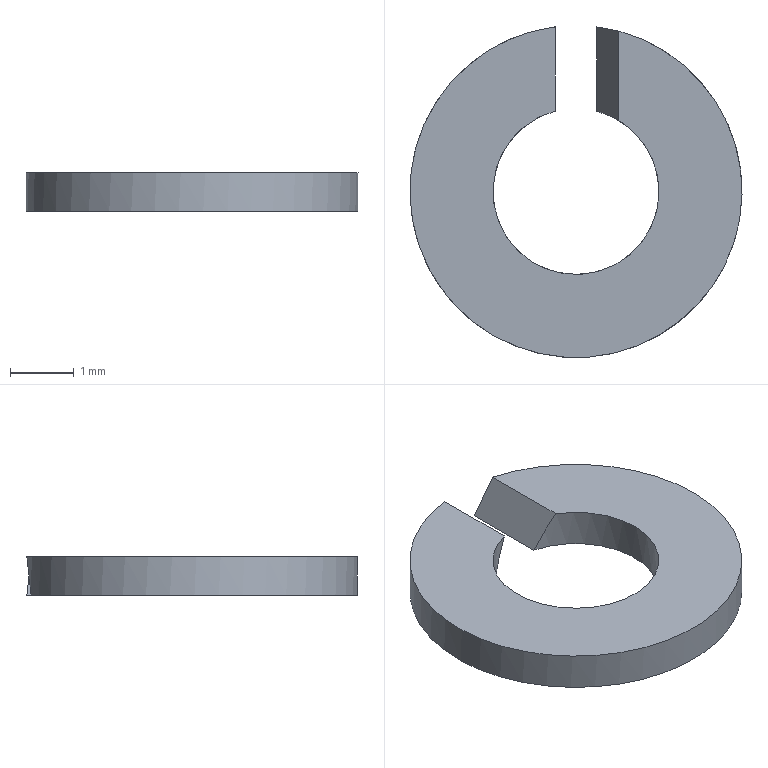Part | STEP file | 1 solid | 6 faces | box 5.2 x 5.179 x 0.6 mm | volume 8.765 mm3 | plane 4 | cylinder 2 | commonest cylinder face diameters 2.6 x1 5.2 x1
STEP:
#1=CARTESIAN_POINT('',(0.,0.,0.));
#2=DIRECTION('',(0.,0.,1.));
#3=DIRECTION('',(1.,0.,0.));
#4=AXIS2_PLACEMENT_3D('',#1,#2,#3);
#5=CARTESIAN_POINT('',(-0.6732,1.112,-0.3));
#6=VERTEX_POINT('',#5);
#7=CARTESIAN_POINT('',(0.3268,1.258,-0.3));
#8=VERTEX_POINT('',#7);
#9=CARTESIAN_POINT('',(0.,0.,-0.3));
#10=DIRECTION('',(0.,0.,1.));
#11=DIRECTION('',(-1.,0.,0.));
#12=AXIS2_PLACEMENT_3D('',#9,#10,#11);
#13=CIRCLE('',#12,1.3);
#14=CARTESIAN_POINT('',(0.,0.,-0.3));
#15=DIRECTION('',(0.,0.,-1.));
#16=DIRECTION('',(-1.,0.,0.));
#17=AXIS2_PLACEMENT_3D('',#14,#15,#16);
#18=PLANE('',#17);
#19=CARTESIAN_POINT('',(1.3,0.));
#20=CARTESIAN_POINT('',(1.3,-2.252));
#21=CARTESIAN_POINT('',(-0.65,-1.126));
#22=CARTESIAN_POINT('',(-2.6,0.));
#23=CARTESIAN_POINT('',(-0.65,1.126));
#24=CARTESIAN_POINT('',(1.3,2.252));
#25=CARTESIAN_POINT('',(1.3,0.));
#26=(BOUNDED_CURVE()B_SPLINE_CURVE(2,(#19,#20,#21,#22,#23,#24,#25),.UNSPECIFIED.,.T.,.F.)B_SPLINE_CURVE_WITH_KNOTS((1,2,2,2,2,1),(-2.094,0.,2.094,4.189,6.283,8.378),.UNSPECIFIED.)CURVE()GEOMETRIC_REPRESENTATION_ITEM()RATIONAL_B_SPLINE_CURVE((1.,0.5,1.,0.5,1.,0.5,1.))REPRESENTATION_ITEM(''));
#27=(GEOMETRIC_REPRESENTATION_CONTEXT(2)PARAMETRIC_REPRESENTATION_CONTEXT()REPRESENTATION_CONTEXT('',''));
#28=DEFINITIONAL_REPRESENTATION('',(#26),#27);
#29=PCURVE('',#18,#28);
#30=CARTESIAN_POINT('',(0.,0.,0.33));
#31=DIRECTION('',(0.,0.,-1.));
#32=DIRECTION('',(-1.,0.,0.));
#33=AXIS2_PLACEMENT_3D('',#30,#31,#32);
#34=CYLINDRICAL_SURFACE('',#33,1.3);
#35=CARTESIAN_POINT('',(12.566,0.63));
#36=DIRECTION('',(-1.,0.));
#37=VECTOR('',#36,1.);
#38=LINE('',#35,#37);
#39=(GEOMETRIC_REPRESENTATION_CONTEXT(2)PARAMETRIC_REPRESENTATION_CONTEXT()REPRESENTATION_CONTEXT('',''));
#40=DEFINITIONAL_REPRESENTATION('',(#38),#39);
#41=PCURVE('',#34,#40);
#42=SURFACE_CURVE('',#13,(#29,#41),.PCURVE_S1.);
#43=EDGE_CURVE('',#6,#8,#42,.T.);
#44=ORIENTED_EDGE('',*,*,#43,.T.);
#45=CARTESIAN_POINT('',(0.3268,2.579,-0.3));
#46=VERTEX_POINT('',#45);
#47=CARTESIAN_POINT('',(0.3268,0.,-0.3));
#48=DIRECTION('',(0.,1.,0.));
#49=VECTOR('',#48,1.);
#50=LINE('',#47,#49);
#51=CARTESIAN_POINT('',(-0.3268,0.));
#52=DIRECTION('',(0.,1.));
#53=VECTOR('',#52,1.);
#54=LINE('',#51,#53);
#55=(GEOMETRIC_REPRESENTATION_CONTEXT(2)PARAMETRIC_REPRESENTATION_CONTEXT()REPRESENTATION_CONTEXT('',''));
#56=DEFINITIONAL_REPRESENTATION('',(#54),#55);
#57=PCURVE('',#18,#56);
#58=CARTESIAN_POINT('',(1.982,0.,2.567));
#59=DIRECTION('',(0.866,0.,-0.5));
#60=DIRECTION('',(-0.5,0.,-0.866));
#61=AXIS2_PLACEMENT_3D('',#58,#59,#60);
#62=PLANE('',#61);
#63=CARTESIAN_POINT('',(3.311,0.));
#64=DIRECTION('',(0.,1.));
#65=VECTOR('',#64,1.);
#66=LINE('',#63,#65);
#67=(GEOMETRIC_REPRESENTATION_CONTEXT(2)PARAMETRIC_REPRESENTATION_CONTEXT()REPRESENTATION_CONTEXT('',''));
#68=DEFINITIONAL_REPRESENTATION('',(#66),#67);
#69=PCURVE('',#62,#68);
#70=SURFACE_CURVE('',#50,(#57,#69),.PCURVE_S1.);
#71=EDGE_CURVE('',#8,#46,#70,.T.);
#72=ORIENTED_EDGE('',*,*,#71,.T.);
#73=CARTESIAN_POINT('',(-0.6732,2.511,-0.3));
#74=VERTEX_POINT('',#73);
#75=CARTESIAN_POINT('',(0.,0.,-0.3));
#76=DIRECTION('',(0.,0.,-1.));
#77=DIRECTION('',(-1.,0.,0.));
#78=AXIS2_PLACEMENT_3D('',#75,#76,#77);
#79=CIRCLE('',#78,2.6);
#80=CARTESIAN_POINT('',(0.,0.));
#81=DIRECTION('',(1.,0.));
#82=AXIS2_PLACEMENT_2D('',#80,#81);
#83=CIRCLE('',#82,2.6);
#84=(GEOMETRIC_REPRESENTATION_CONTEXT(2)PARAMETRIC_REPRESENTATION_CONTEXT()REPRESENTATION_CONTEXT('',''));
#85=DEFINITIONAL_REPRESENTATION('',(#83),#84);
#86=PCURVE('',#18,#85);
#87=CARTESIAN_POINT('',(0.,0.,0.33));
#88=DIRECTION('',(0.,0.,-1.));
#89=DIRECTION('',(-1.,0.,0.));
#90=AXIS2_PLACEMENT_3D('',#87,#88,#89);
#91=CYLINDRICAL_SURFACE('',#90,2.6);
#92=CARTESIAN_POINT('',(0.,0.63));
#93=DIRECTION('',(1.,0.));
#94=VECTOR('',#93,1.);
#95=LINE('',#92,#94);
#96=(GEOMETRIC_REPRESENTATION_CONTEXT(2)PARAMETRIC_REPRESENTATION_CONTEXT()REPRESENTATION_CONTEXT('',''));
#97=DEFINITIONAL_REPRESENTATION('',(#95),#96);
#98=PCURVE('',#91,#97);
#99=SURFACE_CURVE('',#79,(#86,#98),.PCURVE_S1.);
#100=EDGE_CURVE('',#46,#74,#99,.T.);
#101=ORIENTED_EDGE('',*,*,#100,.T.);
#102=CARTESIAN_POINT('',(-0.6732,0.,-0.3));
#103=DIRECTION('',(0.,-1.,0.));
#104=VECTOR('',#103,1.);
#105=LINE('',#102,#104);
#106=CARTESIAN_POINT('',(0.6732,0.));
#107=DIRECTION('',(0.,-1.));
#108=VECTOR('',#107,1.);
#109=LINE('',#106,#108);
#110=(GEOMETRIC_REPRESENTATION_CONTEXT(2)PARAMETRIC_REPRESENTATION_CONTEXT()REPRESENTATION_CONTEXT('',''));
#111=DEFINITIONAL_REPRESENTATION('',(#109),#110);
#112=PCURVE('',#18,#111);
#113=CARTESIAN_POINT('',(-2.232,0.,-3.));
#114=DIRECTION('',(-0.866,0.,0.5));
#115=DIRECTION('',(0.5,0.,0.866));
#116=AXIS2_PLACEMENT_3D('',#113,#114,#115);
#117=PLANE('',#116);
#118=CARTESIAN_POINT('',(3.118,0.));
#119=DIRECTION('',(0.,-1.));
#120=VECTOR('',#119,1.);
#121=LINE('',#118,#120);
#122=(GEOMETRIC_REPRESENTATION_CONTEXT(2)PARAMETRIC_REPRESENTATION_CONTEXT()REPRESENTATION_CONTEXT('',''));
#123=DEFINITIONAL_REPRESENTATION('',(#121),#122);
#124=PCURVE('',#117,#123);
#125=SURFACE_CURVE('',#105,(#112,#124),.PCURVE_S1.);
#126=EDGE_CURVE('',#74,#6,#125,.T.);
#127=ORIENTED_EDGE('',*,*,#126,.T.);
#128=EDGE_LOOP('',(#44,#72,#101,#127));
#129=FACE_BOUND('',#128,.T.);
#130=ADVANCED_FACE('',(#129),#18,.T.);
#131=CARTESIAN_POINT('',(0.6732,1.112,0.3));
#132=VERTEX_POINT('',#131);
#133=CARTESIAN_POINT('',(0.6732,2.511,0.3));
#134=VERTEX_POINT('',#133);
#135=CARTESIAN_POINT('',(0.6732,0.,0.3));
#136=DIRECTION('',(0.,1.,0.));
#137=VECTOR('',#136,1.);
#138=LINE('',#135,#137);
#139=CARTESIAN_POINT('',(2.618,0.));
#140=DIRECTION('',(0.,1.));
#141=VECTOR('',#140,1.);
#142=LINE('',#139,#141);
#143=(GEOMETRIC_REPRESENTATION_CONTEXT(2)PARAMETRIC_REPRESENTATION_CONTEXT()REPRESENTATION_CONTEXT('',''));
#144=DEFINITIONAL_REPRESENTATION('',(#142),#143);
#145=PCURVE('',#62,#144);
#146=CARTESIAN_POINT('',(0.,0.,0.3));
#147=DIRECTION('',(0.,0.,-1.));
#148=DIRECTION('',(-1.,0.,0.));
#149=AXIS2_PLACEMENT_3D('',#146,#147,#148);
#150=PLANE('',#149);
#151=CARTESIAN_POINT('',(-0.6732,0.));
#152=DIRECTION('',(0.,1.));
#153=VECTOR('',#152,1.);
#154=LINE('',#151,#153);
#155=(GEOMETRIC_REPRESENTATION_CONTEXT(2)PARAMETRIC_REPRESENTATION_CONTEXT()REPRESENTATION_CONTEXT('',''));
#156=DEFINITIONAL_REPRESENTATION('',(#154),#155);
#157=PCURVE('',#150,#156);
#158=SURFACE_CURVE('',#138,(#145,#157),.PCURVE_S1.);
#159=EDGE_CURVE('',#132,#134,#158,.T.);
#160=ORIENTED_EDGE('',*,*,#159,.T.);
#161=CARTESIAN_POINT('',(0.3268,2.579,-0.3));
#162=CARTESIAN_POINT('',(0.4437,2.565,-0.09748));
#163=CARTESIAN_POINT('',(0.5594,2.542,0.1028));
#164=CARTESIAN_POINT('',(0.6732,2.511,0.3));
#165=(BOUNDED_CURVE()B_SPLINE_CURVE(3,(#161,#162,#163,#164),.UNSPECIFIED.,.F.,.F.)B_SPLINE_CURVE_WITH_KNOTS((4,4),(1.697,1.833),.PIECEWISE_BEZIER_KNOTS.)CURVE()GEOMETRIC_REPRESENTATION_ITEM()RATIONAL_B_SPLINE_CURVE((1.,0.9985,0.9985,1.))REPRESENTATION_ITEM(''));
#166=CARTESIAN_POINT('',(3.311,2.579));
#167=CARTESIAN_POINT('',(3.077,2.565));
#168=CARTESIAN_POINT('',(2.845,2.542));
#169=CARTESIAN_POINT('',(2.618,2.511));
#170=(BOUNDED_CURVE()B_SPLINE_CURVE(3,(#166,#167,#168,#169),.UNSPECIFIED.,.F.,.F.)B_SPLINE_CURVE_WITH_KNOTS((4,4),(1.697,1.833),.PIECEWISE_BEZIER_KNOTS.)CURVE()GEOMETRIC_REPRESENTATION_ITEM()RATIONAL_B_SPLINE_CURVE((1.,0.9985,0.9985,1.))REPRESENTATION_ITEM(''));
#171=(GEOMETRIC_REPRESENTATION_CONTEXT(2)PARAMETRIC_REPRESENTATION_CONTEXT()REPRESENTATION_CONTEXT('',''));
#172=DEFINITIONAL_REPRESENTATION('',(#170),#171);
#173=PCURVE('',#62,#172);
#174=CARTESIAN_POINT('',(1.697,0.63));
#175=CARTESIAN_POINT('',(1.699,0.6208));
#176=CARTESIAN_POINT('',(1.703,0.6024));
#177=CARTESIAN_POINT('',(1.709,0.5749));
#178=CARTESIAN_POINT('',(1.715,0.5474));
#179=CARTESIAN_POINT('',(1.722,0.5198));
#180=CARTESIAN_POINT('',(1.728,0.4924));
#181=CARTESIAN_POINT('',(1.734,0.4649));
#182=CARTESIAN_POINT('',(1.74,0.4375));
#183=CARTESIAN_POINT('',(1.746,0.41));
#184=CARTESIAN_POINT('',(1.752,0.3827));
#185=CARTESIAN_POINT('',(1.759,0.3553));
#186=CARTESIAN_POINT('',(1.765,0.328));
#187=CARTESIAN_POINT('',(1.771,0.3007));
#188=CARTESIAN_POINT('',(1.777,0.2735));
#189=CARTESIAN_POINT('',(1.783,0.2462));
#190=CARTESIAN_POINT('',(1.789,0.2191));
#191=CARTESIAN_POINT('',(1.796,0.1919));
#192=CARTESIAN_POINT('',(1.802,0.1648));
#193=CARTESIAN_POINT('',(1.808,0.1378));
#194=CARTESIAN_POINT('',(1.814,0.1107));
#195=CARTESIAN_POINT('',(1.82,0.08378));
#196=CARTESIAN_POINT('',(1.827,0.05686));
#197=CARTESIAN_POINT('',(1.831,0.03895));
#198=CARTESIAN_POINT('',(1.833,0.03));
#199=B_SPLINE_CURVE_WITH_KNOTS('',3,(#174,#175,#176,#177,#178,#179,#180,#181,#182,#183,#184,#185,#186,#187,#188,#189,#190,#191,#192,#193,#194,#195,#196,#197,#198),.UNSPECIFIED.,.F.,.F.,(4,1,1,1,1,1,1,1,1,1,1,1,1,1,1,1,1,1,1,1,1,1,4),(1.697,1.703,1.709,1.715,1.722,1.728,1.734,1.74,1.746,1.752,1.759,1.765,1.771,1.777,1.783,1.789,1.796,1.802,1.808,1.814,1.82,1.827,1.833),.QUASI_UNIFORM_KNOTS.);
#200=(GEOMETRIC_REPRESENTATION_CONTEXT(2)PARAMETRIC_REPRESENTATION_CONTEXT()REPRESENTATION_CONTEXT('',''));
#201=DEFINITIONAL_REPRESENTATION('',(#199),#200);
#202=PCURVE('',#91,#201);
#203=SURFACE_CURVE('',#165,(#173,#202),.PCURVE_S1.);
#204=EDGE_CURVE('',#46,#134,#203,.T.);
#205=ORIENTED_EDGE('',*,*,#204,.F.);
#206=ORIENTED_EDGE('',*,*,#71,.F.);
#207=CARTESIAN_POINT('',(0.6732,1.112,0.3));
#208=CARTESIAN_POINT('',(0.5652,1.177,0.113));
#209=CARTESIAN_POINT('',(0.449,1.227,-0.08842));
#210=CARTESIAN_POINT('',(0.3268,1.258,-0.3));
#211=(BOUNDED_CURVE()B_SPLINE_CURVE(3,(#207,#208,#209,#210),.UNSPECIFIED.,.F.,.F.)B_SPLINE_CURVE_WITH_KNOTS((4,4),(4.168,4.458),.PIECEWISE_BEZIER_KNOTS.)CURVE()GEOMETRIC_REPRESENTATION_ITEM()RATIONAL_B_SPLINE_CURVE((1.,0.993,0.993,1.))REPRESENTATION_ITEM(''));
#212=CARTESIAN_POINT('',(2.618,1.112));
#213=CARTESIAN_POINT('',(2.834,1.177));
#214=CARTESIAN_POINT('',(3.066,1.227));
#215=CARTESIAN_POINT('',(3.311,1.258));
#216=(BOUNDED_CURVE()B_SPLINE_CURVE(3,(#212,#213,#214,#215),.UNSPECIFIED.,.F.,.F.)B_SPLINE_CURVE_WITH_KNOTS((4,4),(4.168,4.458),.PIECEWISE_BEZIER_KNOTS.)CURVE()GEOMETRIC_REPRESENTATION_ITEM()RATIONAL_B_SPLINE_CURVE((1.,0.993,0.993,1.))REPRESENTATION_ITEM(''));
#217=(GEOMETRIC_REPRESENTATION_CONTEXT(2)PARAMETRIC_REPRESENTATION_CONTEXT()REPRESENTATION_CONTEXT('',''));
#218=DEFINITIONAL_REPRESENTATION('',(#216),#217);
#219=PCURVE('',#62,#218);
#220=CARTESIAN_POINT('',(2.115,0.03));
#221=CARTESIAN_POINT('',(2.111,0.03844));
#222=CARTESIAN_POINT('',(2.102,0.0554));
#223=CARTESIAN_POINT('',(2.089,0.08105));
#224=CARTESIAN_POINT('',(2.076,0.1069));
#225=CARTESIAN_POINT('',(2.062,0.133));
#226=CARTESIAN_POINT('',(2.049,0.1593));
#227=CARTESIAN_POINT('',(2.036,0.1857));
#228=CARTESIAN_POINT('',(2.023,0.2124));
#229=CARTESIAN_POINT('',(2.01,0.2392));
#230=CARTESIAN_POINT('',(1.996,0.2663));
#231=CARTESIAN_POINT('',(1.983,0.2934));
#232=CARTESIAN_POINT('',(1.97,0.3208));
#233=CARTESIAN_POINT('',(1.957,0.3483));
#234=CARTESIAN_POINT('',(1.944,0.3759));
#235=CARTESIAN_POINT('',(1.93,0.4037));
#236=CARTESIAN_POINT('',(1.917,0.4316));
#237=CARTESIAN_POINT('',(1.904,0.4596));
#238=CARTESIAN_POINT('',(1.891,0.4878));
#239=CARTESIAN_POINT('',(1.878,0.516));
#240=CARTESIAN_POINT('',(1.864,0.5444));
#241=CARTESIAN_POINT('',(1.851,0.5728));
#242=CARTESIAN_POINT('',(1.838,0.6014));
#243=CARTESIAN_POINT('',(1.829,0.6205));
#244=CARTESIAN_POINT('',(1.825,0.63));
#245=B_SPLINE_CURVE_WITH_KNOTS('',3,(#220,#221,#222,#223,#224,#225,#226,#227,#228,#229,#230,#231,#232,#233,#234,#235,#236,#237,#238,#239,#240,#241,#242,#243,#244),.UNSPECIFIED.,.F.,.F.,(4,1,1,1,1,1,1,1,1,1,1,1,1,1,1,1,1,1,1,1,1,1,4),(4.168,4.181,4.194,4.208,4.221,4.234,4.247,4.26,4.274,4.287,4.3,4.313,4.326,4.34,4.353,4.366,4.379,4.392,4.406,4.419,4.432,4.445,4.458),.QUASI_UNIFORM_KNOTS.);
#246=(GEOMETRIC_REPRESENTATION_CONTEXT(2)PARAMETRIC_REPRESENTATION_CONTEXT()REPRESENTATION_CONTEXT('',''));
#247=DEFINITIONAL_REPRESENTATION('',(#245),#246);
#248=PCURVE('',#34,#247);
#249=SURFACE_CURVE('',#211,(#219,#248),.PCURVE_S1.);
#250=EDGE_CURVE('',#132,#8,#249,.T.);
#251=ORIENTED_EDGE('',*,*,#250,.F.);
#252=EDGE_LOOP('',(#160,#205,#206,#251));
#253=FACE_BOUND('',#252,.T.);
#254=ADVANCED_FACE('',(#253),#62,.F.);
#255=CARTESIAN_POINT('',(-0.3268,1.258,0.3));
#256=VERTEX_POINT('',#255);
#257=CARTESIAN_POINT('',(-0.3268,1.258,0.3));
#258=CARTESIAN_POINT('',(-0.449,1.227,0.08842));
#259=CARTESIAN_POINT('',(-0.5652,1.177,-0.113));
#260=CARTESIAN_POINT('',(-0.6732,1.112,-0.3));
#261=(BOUNDED_CURVE()B_SPLINE_CURVE(3,(#257,#258,#259,#260),.UNSPECIFIED.,.F.,.F.)B_SPLINE_CURVE_WITH_KNOTS((4,4),(4.966,5.257),.PIECEWISE_BEZIER_KNOTS.)CURVE()GEOMETRIC_REPRESENTATION_ITEM()RATIONAL_B_SPLINE_CURVE((1.,0.993,0.993,1.))REPRESENTATION_ITEM(''));
#262=CARTESIAN_POINT('',(7.6,0.03));
#263=CARTESIAN_POINT('',(7.595,0.03955));
#264=CARTESIAN_POINT('',(7.587,0.05863));
#265=CARTESIAN_POINT('',(7.574,0.08716));
#266=CARTESIAN_POINT('',(7.56,0.1156));
#267=CARTESIAN_POINT('',(7.547,0.144));
#268=CARTESIAN_POINT('',(7.534,0.1722));
#269=CARTESIAN_POINT('',(7.521,0.2004));
#270=CARTESIAN_POINT('',(7.508,0.2284));
#271=CARTESIAN_POINT('',(7.494,0.2563));
#272=CARTESIAN_POINT('',(7.481,0.2841));
#273=CARTESIAN_POINT('',(7.468,0.3117));
#274=CARTESIAN_POINT('',(7.455,0.3392));
#275=CARTESIAN_POINT('',(7.442,0.3666));
#276=CARTESIAN_POINT('',(7.428,0.3937));
#277=CARTESIAN_POINT('',(7.415,0.4208));
#278=CARTESIAN_POINT('',(7.402,0.4476));
#279=CARTESIAN_POINT('',(7.389,0.4743));
#280=CARTESIAN_POINT('',(7.376,0.5007));
#281=CARTESIAN_POINT('',(7.362,0.527));
#282=CARTESIAN_POINT('',(7.349,0.5531));
#283=CARTESIAN_POINT('',(7.336,0.5789));
#284=CARTESIAN_POINT('',(7.323,0.6046));
#285=CARTESIAN_POINT('',(7.314,0.6216));
#286=CARTESIAN_POINT('',(7.31,0.63));
#287=B_SPLINE_CURVE_WITH_KNOTS('',3,(#262,#263,#264,#265,#266,#267,#268,#269,#270,#271,#272,#273,#274,#275,#276,#277,#278,#279,#280,#281,#282,#283,#284,#285,#286),.UNSPECIFIED.,.F.,.F.,(4,1,1,1,1,1,1,1,1,1,1,1,1,1,1,1,1,1,1,1,1,1,4),(4.966,4.98,4.993,5.006,5.019,5.032,5.046,5.059,5.072,5.085,5.098,5.112,5.125,5.138,5.151,5.164,5.178,5.191,5.204,5.217,5.23,5.244,5.257),.QUASI_UNIFORM_KNOTS.);
#288=(GEOMETRIC_REPRESENTATION_CONTEXT(2)PARAMETRIC_REPRESENTATION_CONTEXT()REPRESENTATION_CONTEXT('',''));
#289=DEFINITIONAL_REPRESENTATION('',(#287),#288);
#290=PCURVE('',#34,#289);
#291=CARTESIAN_POINT('',(3.811,1.258));
#292=CARTESIAN_POINT('',(3.566,1.227));
#293=CARTESIAN_POINT('',(3.334,1.177));
#294=CARTESIAN_POINT('',(3.118,1.112));
#295=(BOUNDED_CURVE()B_SPLINE_CURVE(3,(#291,#292,#293,#294),.UNSPECIFIED.,.F.,.F.)B_SPLINE_CURVE_WITH_KNOTS((4,4),(4.966,5.257),.PIECEWISE_BEZIER_KNOTS.)CURVE()GEOMETRIC_REPRESENTATION_ITEM()RATIONAL_B_SPLINE_CURVE((1.,0.993,0.993,1.))REPRESENTATION_ITEM(''));
#296=(GEOMETRIC_REPRESENTATION_CONTEXT(2)PARAMETRIC_REPRESENTATION_CONTEXT()REPRESENTATION_CONTEXT('',''));
#297=DEFINITIONAL_REPRESENTATION('',(#295),#296);
#298=PCURVE('',#117,#297);
#299=SURFACE_CURVE('',#261,(#290,#298),.PCURVE_S1.);
#300=EDGE_CURVE('',#256,#6,#299,.T.);
#301=ORIENTED_EDGE('',*,*,#300,.T.);
#302=ORIENTED_EDGE('',*,*,#43,.T.);
#303=ORIENTED_EDGE('',*,*,#250,.F.);
#304=CARTESIAN_POINT('',(0.,0.,0.3));
#305=DIRECTION('',(0.,0.,-1.));
#306=DIRECTION('',(-1.,0.,0.));
#307=AXIS2_PLACEMENT_3D('',#304,#305,#306);
#308=CIRCLE('',#307,1.3);
#309=CARTESIAN_POINT('',(0.,0.03));
#310=DIRECTION('',(1.,0.));
#311=VECTOR('',#310,1.);
#312=LINE('',#309,#311);
#313=(GEOMETRIC_REPRESENTATION_CONTEXT(2)PARAMETRIC_REPRESENTATION_CONTEXT()REPRESENTATION_CONTEXT('',''));
#314=DEFINITIONAL_REPRESENTATION('',(#312),#313);
#315=PCURVE('',#34,#314);
#316=CARTESIAN_POINT('',(0.,0.));
#317=DIRECTION('',(1.,0.));
#318=AXIS2_PLACEMENT_2D('',#316,#317);
#319=CIRCLE('',#318,1.3);
#320=(GEOMETRIC_REPRESENTATION_CONTEXT(2)PARAMETRIC_REPRESENTATION_CONTEXT()REPRESENTATION_CONTEXT('',''));
#321=DEFINITIONAL_REPRESENTATION('',(#319),#320);
#322=PCURVE('',#150,#321);
#323=SURFACE_CURVE('',#308,(#315,#322),.PCURVE_S1.);
#324=EDGE_CURVE('',#132,#256,#323,.T.);
#325=ORIENTED_EDGE('',*,*,#324,.T.);
#326=EDGE_LOOP('',(#301,#302,#303,#325));
#327=FACE_BOUND('',#326,.F.);
#328=ADVANCED_FACE('',(#327),#34,.F.);
#329=CARTESIAN_POINT('',(-0.3268,2.579,0.3));
#330=VERTEX_POINT('',#329);
#331=CARTESIAN_POINT('',(-0.3268,2.579,0.3));
#332=CARTESIAN_POINT('',(-0.4437,2.565,0.09748));
#333=CARTESIAN_POINT('',(-0.5594,2.542,-0.1028));
#334=CARTESIAN_POINT('',(-0.6732,2.511,-0.3));
#335=(BOUNDED_CURVE()B_SPLINE_CURVE(3,(#331,#332,#333,#334),.UNSPECIFIED.,.F.,.F.)B_SPLINE_CURVE_WITH_KNOTS((4,4),(4.838,4.974),.PIECEWISE_BEZIER_KNOTS.)CURVE()GEOMETRIC_REPRESENTATION_ITEM()RATIONAL_B_SPLINE_CURVE((1.,0.9985,0.9985,1.))REPRESENTATION_ITEM(''));
#336=CARTESIAN_POINT('',(3.811,2.579));
#337=CARTESIAN_POINT('',(3.577,2.565));
#338=CARTESIAN_POINT('',(3.345,2.542));
#339=CARTESIAN_POINT('',(3.118,2.511));
#340=(BOUNDED_CURVE()B_SPLINE_CURVE(3,(#336,#337,#338,#339),.UNSPECIFIED.,.F.,.F.)B_SPLINE_CURVE_WITH_KNOTS((4,4),(4.838,4.974),.PIECEWISE_BEZIER_KNOTS.)CURVE()GEOMETRIC_REPRESENTATION_ITEM()RATIONAL_B_SPLINE_CURVE((1.,0.9985,0.9985,1.))REPRESENTATION_ITEM(''));
#341=(GEOMETRIC_REPRESENTATION_CONTEXT(2)PARAMETRIC_REPRESENTATION_CONTEXT()REPRESENTATION_CONTEXT('',''));
#342=DEFINITIONAL_REPRESENTATION('',(#340),#341);
#343=PCURVE('',#117,#342);
#344=CARTESIAN_POINT('',(7.728,0.03));
#345=CARTESIAN_POINT('',(7.726,0.03919));
#346=CARTESIAN_POINT('',(7.722,0.05757));
#347=CARTESIAN_POINT('',(7.716,0.08512));
#348=CARTESIAN_POINT('',(7.709,0.1126));
#349=CARTESIAN_POINT('',(7.703,0.1402));
#350=CARTESIAN_POINT('',(7.697,0.1676));
#351=CARTESIAN_POINT('',(7.691,0.1951));
#352=CARTESIAN_POINT('',(7.685,0.2225));
#353=CARTESIAN_POINT('',(7.679,0.25));
#354=CARTESIAN_POINT('',(7.672,0.2773));
#355=CARTESIAN_POINT('',(7.666,0.3047));
#356=CARTESIAN_POINT('',(7.66,0.332));
#357=CARTESIAN_POINT('',(7.654,0.3593));
#358=CARTESIAN_POINT('',(7.648,0.3865));
#359=CARTESIAN_POINT('',(7.641,0.4138));
#360=CARTESIAN_POINT('',(7.635,0.4409));
#361=CARTESIAN_POINT('',(7.629,0.4681));
#362=CARTESIAN_POINT('',(7.623,0.4952));
#363=CARTESIAN_POINT('',(7.617,0.5222));
#364=CARTESIAN_POINT('',(7.611,0.5493));
#365=CARTESIAN_POINT('',(7.604,0.5762));
#366=CARTESIAN_POINT('',(7.598,0.6031));
#367=CARTESIAN_POINT('',(7.594,0.6211));
#368=CARTESIAN_POINT('',(7.592,0.63));
#369=B_SPLINE_CURVE_WITH_KNOTS('',3,(#344,#345,#346,#347,#348,#349,#350,#351,#352,#353,#354,#355,#356,#357,#358,#359,#360,#361,#362,#363,#364,#365,#366,#367,#368),.UNSPECIFIED.,.F.,.F.,(4,1,1,1,1,1,1,1,1,1,1,1,1,1,1,1,1,1,1,1,1,1,4),(4.838,4.845,4.851,4.857,4.863,4.869,4.875,4.882,4.888,4.894,4.9,4.906,4.913,4.919,4.925,4.931,4.937,4.943,4.95,4.956,4.962,4.968,4.974),.QUASI_UNIFORM_KNOTS.);
#370=(GEOMETRIC_REPRESENTATION_CONTEXT(2)PARAMETRIC_REPRESENTATION_CONTEXT()REPRESENTATION_CONTEXT('',''));
#371=DEFINITIONAL_REPRESENTATION('',(#369),#370);
#372=PCURVE('',#91,#371);
#373=SURFACE_CURVE('',#335,(#343,#372),.PCURVE_S1.);
#374=EDGE_CURVE('',#330,#74,#373,.T.);
#375=ORIENTED_EDGE('',*,*,#374,.F.);
#376=CARTESIAN_POINT('',(-0.3268,0.,0.3));
#377=DIRECTION('',(0.,1.,0.));
#378=VECTOR('',#377,1.);
#379=LINE('',#376,#378);
#380=CARTESIAN_POINT('',(3.811,0.));
#381=DIRECTION('',(0.,1.));
#382=VECTOR('',#381,1.);
#383=LINE('',#380,#382);
#384=(GEOMETRIC_REPRESENTATION_CONTEXT(2)PARAMETRIC_REPRESENTATION_CONTEXT()REPRESENTATION_CONTEXT('',''));
#385=DEFINITIONAL_REPRESENTATION('',(#383),#384);
#386=PCURVE('',#117,#385);
#387=CARTESIAN_POINT('',(0.3268,0.));
#388=DIRECTION('',(0.,1.));
#389=VECTOR('',#388,1.);
#390=LINE('',#387,#389);
#391=(GEOMETRIC_REPRESENTATION_CONTEXT(2)PARAMETRIC_REPRESENTATION_CONTEXT()REPRESENTATION_CONTEXT('',''));
#392=DEFINITIONAL_REPRESENTATION('',(#390),#391);
#393=PCURVE('',#150,#392);
#394=SURFACE_CURVE('',#379,(#386,#393),.PCURVE_S1.);
#395=EDGE_CURVE('',#256,#330,#394,.T.);
#396=ORIENTED_EDGE('',*,*,#395,.F.);
#397=ORIENTED_EDGE('',*,*,#300,.T.);
#398=ORIENTED_EDGE('',*,*,#126,.F.);
#399=EDGE_LOOP('',(#375,#396,#397,#398));
#400=FACE_BOUND('',#399,.T.);
#401=ADVANCED_FACE('',(#400),#117,.F.);
#402=ORIENTED_EDGE('',*,*,#374,.T.);
#403=ORIENTED_EDGE('',*,*,#100,.F.);
#404=ORIENTED_EDGE('',*,*,#204,.T.);
#405=CARTESIAN_POINT('',(0.,0.,0.3));
#406=DIRECTION('',(0.,0.,-1.));
#407=DIRECTION('',(-1.,0.,0.));
#408=AXIS2_PLACEMENT_3D('',#405,#406,#407);
#409=CIRCLE('',#408,2.6);
#410=CARTESIAN_POINT('',(0.,0.03));
#411=DIRECTION('',(1.,0.));
#412=VECTOR('',#411,1.);
#413=LINE('',#410,#412);
#414=(GEOMETRIC_REPRESENTATION_CONTEXT(2)PARAMETRIC_REPRESENTATION_CONTEXT()REPRESENTATION_CONTEXT('',''));
#415=DEFINITIONAL_REPRESENTATION('',(#413),#414);
#416=PCURVE('',#91,#415);
#417=CARTESIAN_POINT('',(0.,0.));
#418=DIRECTION('',(1.,0.));
#419=AXIS2_PLACEMENT_2D('',#417,#418);
#420=CIRCLE('',#419,2.6);
#421=(GEOMETRIC_REPRESENTATION_CONTEXT(2)PARAMETRIC_REPRESENTATION_CONTEXT()REPRESENTATION_CONTEXT('',''));
#422=DEFINITIONAL_REPRESENTATION('',(#420),#421);
#423=PCURVE('',#150,#422);
#424=SURFACE_CURVE('',#409,(#416,#423),.PCURVE_S1.);
#425=EDGE_CURVE('',#134,#330,#424,.T.);
#426=ORIENTED_EDGE('',*,*,#425,.T.);
#427=EDGE_LOOP('',(#402,#403,#404,#426));
#428=FACE_BOUND('',#427,.T.);
#429=ADVANCED_FACE('',(#428),#91,.T.);
#430=ORIENTED_EDGE('',*,*,#159,.F.);
#431=ORIENTED_EDGE('',*,*,#324,.T.);
#432=ORIENTED_EDGE('',*,*,#395,.T.);
#433=ORIENTED_EDGE('',*,*,#425,.F.);
#434=EDGE_LOOP('',(#430,#431,#432,#433));
#435=FACE_BOUND('',#434,.T.);
#436=ADVANCED_FACE('',(#435),#150,.F.);
#437=CLOSED_SHELL('',(#130,#254,#328,#401,#429,#436));
#438=MANIFOLD_SOLID_BREP('',#437);
#439=(LENGTH_UNIT()NAMED_UNIT(*)SI_UNIT(.MILLI.,.METRE.));
#440=UNCERTAINTY_MEASURE_WITH_UNIT(LENGTH_MEASURE(0.0000001),#439,'','');
#441=(NAMED_UNIT(*)PLANE_ANGLE_UNIT()SI_UNIT($,.RADIAN.));
#442=(NAMED_UNIT(*)SI_UNIT($,.STERADIAN.)SOLID_ANGLE_UNIT());
#443=(GEOMETRIC_REPRESENTATION_CONTEXT(3)GLOBAL_UNCERTAINTY_ASSIGNED_CONTEXT((#440))GLOBAL_UNIT_ASSIGNED_CONTEXT((#439,#441,#442))REPRESENTATION_CONTEXT('',''));
#444=ADVANCED_BREP_SHAPE_REPRESENTATION('',(#4,#438),#443);